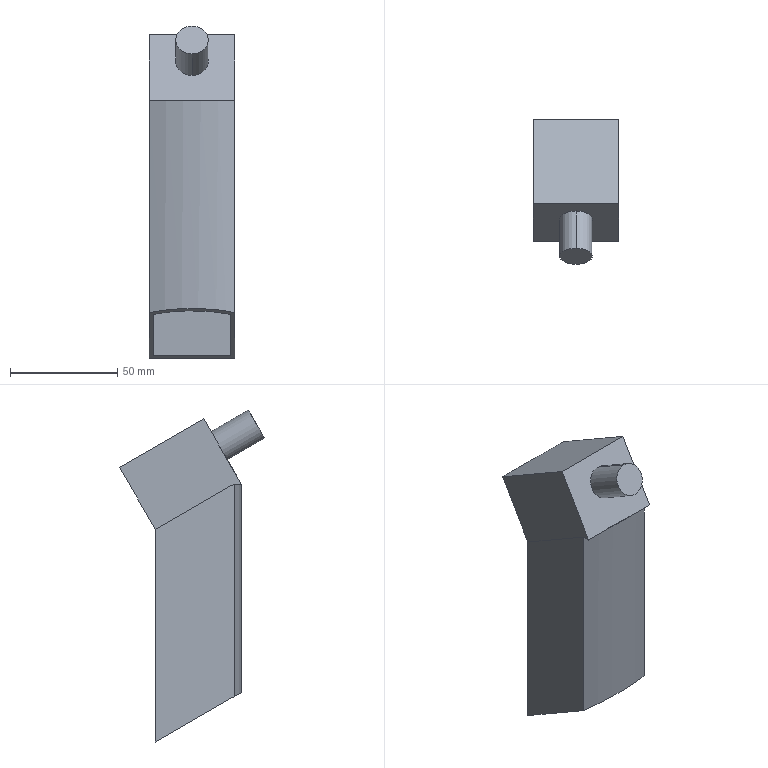Part | NX | 2 solids | 28 faces | box 40 x 67.338 x 154.471 mm | volume 46471 mm3 | plane 24 | cylinder 4 | commonest cylinder face diameters 15 x2 116 x1 120 x1
STEP:
#1=CARTESIAN_POINT('',(-12.806,-56.569,120.));
#2=VERTEX_POINT('',#1);
#3=CARTESIAN_POINT('',(-20.,-56.569,120.));
#4=VERTEX_POINT('',#3);
#5=CARTESIAN_POINT('',(25.,-56.569,120.));
#6=DIRECTION('',(-1.,0.,0.));
#7=VECTOR('',#6,1.);
#8=LINE('',#5,#7);
#9=EDGE_CURVE('',#2,#4,#8,.T.);
#10=ORIENTED_EDGE('',*,*,#9,.T.);
#11=CARTESIAN_POINT('',(20.,-56.569,120.));
#12=VERTEX_POINT('',#11);
#13=CARTESIAN_POINT('',(0.,0.,120.));
#14=DIRECTION('',(0.,0.,1.));
#15=DIRECTION('',(1.,0.,0.));
#16=AXIS2_PLACEMENT_3D('',#13,#14,#15);
#17=CIRCLE('',#16,60.);
#18=EDGE_CURVE('',#4,#12,#17,.T.);
#19=ORIENTED_EDGE('',*,*,#18,.T.);
#20=CARTESIAN_POINT('',(12.806,-56.569,120.));
#21=VERTEX_POINT('',#20);
#22=CARTESIAN_POINT('',(25.,-56.569,120.));
#23=DIRECTION('',(-1.,0.,0.));
#24=VECTOR('',#23,1.);
#25=LINE('',#22,#24);
#26=EDGE_CURVE('',#12,#21,#25,.T.);
#27=ORIENTED_EDGE('',*,*,#26,.T.);
#28=CARTESIAN_POINT('',(0.,0.,120.));
#29=DIRECTION('',(0.,0.,1.));
#30=DIRECTION('',(1.,0.,0.));
#31=AXIS2_PLACEMENT_3D('',#28,#29,#30);
#32=CIRCLE('',#31,58.);
#33=EDGE_CURVE('',#2,#21,#32,.T.);
#34=ORIENTED_EDGE('',*,*,#33,.F.);
#35=EDGE_LOOP('',(#10,#19,#27,#34));
#36=FACE_OUTER_BOUND('',#35,.T.);
#37=CARTESIAN_POINT('',(0.,0.,120.));
#38=DIRECTION('',(0.,0.,1.));
#39=DIRECTION('',(1.,0.,0.));
#40=AXIS2_PLACEMENT_3D('',#37,#38,#39);
#41=PLANE('',#40);
#42=ADVANCED_FACE('',(#36),#41,.T.);
#43=CARTESIAN_POINT('',(-20.,-56.569,21.113));
#44=VERTEX_POINT('',#43);
#45=CARTESIAN_POINT('',(-20.,-56.569,120.));
#46=DIRECTION('',(0.,0.,-1.));
#47=VECTOR('',#46,1.);
#48=LINE('',#45,#47);
#49=EDGE_CURVE('',#4,#44,#48,.T.);
#50=ORIENTED_EDGE('',*,*,#49,.T.);
#51=CARTESIAN_POINT('',(20.,-56.569,21.113));
#52=VERTEX_POINT('',#51);
#53=CARTESIAN_POINT('',(-20.,-56.569,21.113));
#54=CARTESIAN_POINT('',(-6.931,-61.189,23.781));
#55=CARTESIAN_POINT('',(6.931,-61.189,23.781));
#56=CARTESIAN_POINT('',(20.,-56.569,21.113));
#57=(BOUNDED_CURVE()B_SPLINE_CURVE(3,(#53,#54,#55,#56),.UNSPECIFIED.,.F.,.F.)B_SPLINE_CURVE_WITH_KNOTS((4,4),(0.,1.),.UNSPECIFIED.)CURVE()GEOMETRIC_REPRESENTATION_ITEM()RATIONAL_B_SPLINE_CURVE((1.,0.9619,0.9619,1.))REPRESENTATION_ITEM(''));
#58=EDGE_CURVE('',#44,#52,#57,.T.);
#59=ORIENTED_EDGE('',*,*,#58,.T.);
#60=CARTESIAN_POINT('',(20.,-56.569,120.));
#61=DIRECTION('',(0.,0.,-1.));
#62=VECTOR('',#61,1.);
#63=LINE('',#60,#62);
#64=EDGE_CURVE('',#12,#52,#63,.T.);
#65=ORIENTED_EDGE('',*,*,#64,.F.);
#66=ORIENTED_EDGE('',*,*,#18,.F.);
#67=EDGE_LOOP('',(#50,#59,#65,#66));
#68=FACE_OUTER_BOUND('',#67,.T.);
#69=CARTESIAN_POINT('',(0.,0.,120.));
#70=DIRECTION('',(0.,0.,-1.));
#71=DIRECTION('',(-1.,0.,0.));
#72=AXIS2_PLACEMENT_3D('',#69,#70,#71);
#73=CYLINDRICAL_SURFACE('',#72,60.);
#74=ADVANCED_FACE('',(#68),#73,.T.);
#75=CARTESIAN_POINT('',(20.,-20.,98.887));
#76=VERTEX_POINT('',#75);
#77=CARTESIAN_POINT('',(20.,-20.,0.));
#78=VERTEX_POINT('',#77);
#79=CARTESIAN_POINT('',(20.,-20.,120.));
#80=DIRECTION('',(0.,0.,-1.));
#81=VECTOR('',#80,1.);
#82=LINE('',#79,#81);
#83=EDGE_CURVE('',#76,#78,#82,.T.);
#84=ORIENTED_EDGE('',*,*,#83,.F.);
#85=CARTESIAN_POINT('',(20.,-56.569,120.));
#86=DIRECTION('',(0.,-0.866,0.5));
#87=VECTOR('',#86,1.);
#88=LINE('',#85,#87);
#89=EDGE_CURVE('',#76,#12,#88,.T.);
#90=ORIENTED_EDGE('',*,*,#89,.T.);
#91=ORIENTED_EDGE('',*,*,#64,.T.);
#92=CARTESIAN_POINT('',(20.,-60.,23.094));
#93=DIRECTION('',(0.,0.866,-0.5));
#94=VECTOR('',#93,1.);
#95=LINE('',#92,#94);
#96=EDGE_CURVE('',#52,#78,#95,.T.);
#97=ORIENTED_EDGE('',*,*,#96,.T.);
#98=EDGE_LOOP('',(#84,#90,#91,#97));
#99=FACE_OUTER_BOUND('',#98,.T.);
#100=CARTESIAN_POINT('',(20.,-56.569,120.));
#101=DIRECTION('',(-1.,0.,0.));
#102=DIRECTION('',(0.,0.,1.));
#103=AXIS2_PLACEMENT_3D('',#100,#101,#102);
#104=PLANE('',#103);
#105=ADVANCED_FACE('',(#99),#104,.F.);
#106=CARTESIAN_POINT('',(-20.,-20.,98.887));
#107=VERTEX_POINT('',#106);
#108=CARTESIAN_POINT('',(-20.,-20.,0.));
#109=VERTEX_POINT('',#108);
#110=CARTESIAN_POINT('',(-20.,-20.,120.));
#111=DIRECTION('',(0.,0.,-1.));
#112=VECTOR('',#111,1.);
#113=LINE('',#110,#112);
#114=EDGE_CURVE('',#107,#109,#113,.T.);
#115=ORIENTED_EDGE('',*,*,#114,.F.);
#116=CARTESIAN_POINT('',(25.,-20.,98.887));
#117=DIRECTION('',(-1.,0.,0.));
#118=VECTOR('',#117,1.);
#119=LINE('',#116,#118);
#120=EDGE_CURVE('',#76,#107,#119,.T.);
#121=ORIENTED_EDGE('',*,*,#120,.F.);
#122=ORIENTED_EDGE('',*,*,#83,.T.);
#123=CARTESIAN_POINT('',(-20.,-20.,0.));
#124=DIRECTION('',(-1.,0.,0.));
#125=VECTOR('',#124,1.);
#126=LINE('',#123,#125);
#127=EDGE_CURVE('',#78,#109,#126,.T.);
#128=ORIENTED_EDGE('',*,*,#127,.T.);
#129=EDGE_LOOP('',(#115,#121,#122,#128));
#130=FACE_OUTER_BOUND('',#129,.T.);
#131=CARTESIAN_POINT('',(-20.,-20.,120.));
#132=DIRECTION('',(0.,-1.,0.));
#133=DIRECTION('',(0.,0.,-1.));
#134=AXIS2_PLACEMENT_3D('',#131,#132,#133);
#135=PLANE('',#134);
#136=ADVANCED_FACE('',(#130),#135,.F.);
#137=ORIENTED_EDGE('',*,*,#49,.F.);
#138=CARTESIAN_POINT('',(-20.,-56.569,120.));
#139=DIRECTION('',(0.,-0.866,0.5));
#140=VECTOR('',#139,1.);
#141=LINE('',#138,#140);
#142=EDGE_CURVE('',#107,#4,#141,.T.);
#143=ORIENTED_EDGE('',*,*,#142,.F.);
#144=ORIENTED_EDGE('',*,*,#114,.T.);
#145=CARTESIAN_POINT('',(-20.,-60.,23.094));
#146=DIRECTION('',(0.,0.866,-0.5));
#147=VECTOR('',#146,1.);
#148=LINE('',#145,#147);
#149=EDGE_CURVE('',#44,#109,#148,.T.);
#150=ORIENTED_EDGE('',*,*,#149,.F.);
#151=EDGE_LOOP('',(#137,#143,#144,#150));
#152=FACE_OUTER_BOUND('',#151,.T.);
#153=CARTESIAN_POINT('',(-20.,-56.569,120.));
#154=DIRECTION('',(1.,0.,0.));
#155=DIRECTION('',(0.,0.,-1.));
#156=AXIS2_PLACEMENT_3D('',#153,#154,#155);
#157=PLANE('',#156);
#158=ADVANCED_FACE('',(#152),#157,.F.);
#159=CARTESIAN_POINT('',(-18.,-55.136,119.173));
#160=VERTEX_POINT('',#159);
#161=CARTESIAN_POINT('',(-18.,-22.,100.042));
#162=VERTEX_POINT('',#161);
#163=CARTESIAN_POINT('',(-18.,-55.494,119.38));
#164=DIRECTION('',(0.,0.866,-0.5));
#165=VECTOR('',#164,1.);
#166=LINE('',#163,#165);
#167=EDGE_CURVE('',#160,#162,#166,.T.);
#168=ORIENTED_EDGE('',*,*,#167,.F.);
#169=CARTESIAN_POINT('',(-18.,-55.136,20.286));
#170=VERTEX_POINT('',#169);
#171=CARTESIAN_POINT('',(-18.,-55.136,120.));
#172=DIRECTION('',(0.,0.,-1.));
#173=VECTOR('',#172,1.);
#174=LINE('',#171,#173);
#175=EDGE_CURVE('',#160,#170,#174,.T.);
#176=ORIENTED_EDGE('',*,*,#175,.T.);
#177=CARTESIAN_POINT('',(-18.,-22.,1.155));
#178=VERTEX_POINT('',#177);
#179=CARTESIAN_POINT('',(-18.,-98.314,45.214));
#180=DIRECTION('',(0.,-0.866,0.5));
#181=VECTOR('',#180,1.);
#182=LINE('',#179,#181);
#183=EDGE_CURVE('',#178,#170,#182,.T.);
#184=ORIENTED_EDGE('',*,*,#183,.F.);
#185=CARTESIAN_POINT('',(-18.,-22.,120.));
#186=DIRECTION('',(0.,0.,-1.));
#187=VECTOR('',#186,1.);
#188=LINE('',#185,#187);
#189=EDGE_CURVE('',#162,#178,#188,.T.);
#190=ORIENTED_EDGE('',*,*,#189,.F.);
#191=EDGE_LOOP('',(#168,#176,#184,#190));
#192=FACE_OUTER_BOUND('',#191,.T.);
#193=CARTESIAN_POINT('',(-18.,-55.136,120.));
#194=DIRECTION('',(1.,0.,0.));
#195=DIRECTION('',(0.,1.,0.));
#196=AXIS2_PLACEMENT_3D('',#193,#194,#195);
#197=PLANE('',#196);
#198=ADVANCED_FACE('',(#192),#197,.T.);
#199=CARTESIAN_POINT('',(18.,-55.136,119.173));
#200=VERTEX_POINT('',#199);
#201=CARTESIAN_POINT('',(18.,-55.136,119.173));
#202=CARTESIAN_POINT('',(16.292,-55.694,119.495));
#203=CARTESIAN_POINT('',(14.559,-56.172,119.771));
#204=CARTESIAN_POINT('',(12.806,-56.569,120.));
#205=(BOUNDED_CURVE()B_SPLINE_CURVE(3,(#201,#202,#203,#204),.UNSPECIFIED.,.F.,.F.)B_SPLINE_CURVE_WITH_KNOTS((4,4),(0.,1.),.UNSPECIFIED.)CURVE()GEOMETRIC_REPRESENTATION_ITEM()RATIONAL_B_SPLINE_CURVE((1.,0.9993,0.9993,1.))REPRESENTATION_ITEM(''));
#206=EDGE_CURVE('',#200,#21,#205,.T.);
#207=ORIENTED_EDGE('',*,*,#206,.F.);
#208=CARTESIAN_POINT('',(18.,-55.136,20.286));
#209=VERTEX_POINT('',#208);
#210=CARTESIAN_POINT('',(18.,-55.136,120.));
#211=DIRECTION('',(0.,0.,-1.));
#212=VECTOR('',#211,1.);
#213=LINE('',#210,#212);
#214=EDGE_CURVE('',#200,#209,#213,.T.);
#215=ORIENTED_EDGE('',*,*,#214,.T.);
#216=CARTESIAN_POINT('',(-18.,-55.136,20.286));
#217=CARTESIAN_POINT('',(-6.204,-58.987,22.509));
#218=CARTESIAN_POINT('',(6.204,-58.987,22.509));
#219=CARTESIAN_POINT('',(18.,-55.136,20.286));
#220=(BOUNDED_CURVE()B_SPLINE_CURVE(3,(#216,#217,#218,#219),.UNSPECIFIED.,.F.,.F.)B_SPLINE_CURVE_WITH_KNOTS((4,4),(0.,1.),.UNSPECIFIED.)CURVE()GEOMETRIC_REPRESENTATION_ITEM()RATIONAL_B_SPLINE_CURVE((1.,0.9671,0.9671,1.))REPRESENTATION_ITEM(''));
#221=EDGE_CURVE('',#170,#209,#220,.T.);
#222=ORIENTED_EDGE('',*,*,#221,.F.);
#223=ORIENTED_EDGE('',*,*,#175,.F.);
#224=CARTESIAN_POINT('',(-12.806,-56.569,120.));
#225=CARTESIAN_POINT('',(-14.559,-56.172,119.771));
#226=CARTESIAN_POINT('',(-16.292,-55.694,119.495));
#227=CARTESIAN_POINT('',(-18.,-55.136,119.173));
#228=(BOUNDED_CURVE()B_SPLINE_CURVE(3,(#224,#225,#226,#227),.UNSPECIFIED.,.F.,.F.)B_SPLINE_CURVE_WITH_KNOTS((4,4),(0.,1.),.UNSPECIFIED.)CURVE()GEOMETRIC_REPRESENTATION_ITEM()RATIONAL_B_SPLINE_CURVE((1.,0.9993,0.9993,1.))REPRESENTATION_ITEM(''));
#229=EDGE_CURVE('',#2,#160,#228,.T.);
#230=ORIENTED_EDGE('',*,*,#229,.F.);
#231=ORIENTED_EDGE('',*,*,#33,.T.);
#232=EDGE_LOOP('',(#207,#215,#222,#223,#230,#231));
#233=FACE_OUTER_BOUND('',#232,.T.);
#234=CARTESIAN_POINT('',(0.,0.,120.));
#235=DIRECTION('',(0.,0.,-1.));
#236=DIRECTION('',(-1.,0.,0.));
#237=AXIS2_PLACEMENT_3D('',#234,#235,#236);
#238=CYLINDRICAL_SURFACE('',#237,58.);
#239=ADVANCED_FACE('',(#233),#238,.F.);
#240=CARTESIAN_POINT('',(18.,-22.,100.042));
#241=VERTEX_POINT('',#240);
#242=CARTESIAN_POINT('',(18.,-55.494,119.38));
#243=DIRECTION('',(0.,-0.866,0.5));
#244=VECTOR('',#243,1.);
#245=LINE('',#242,#244);
#246=EDGE_CURVE('',#241,#200,#245,.T.);
#247=ORIENTED_EDGE('',*,*,#246,.F.);
#248=CARTESIAN_POINT('',(18.,-22.,1.155));
#249=VERTEX_POINT('',#248);
#250=CARTESIAN_POINT('',(18.,-22.,120.));
#251=DIRECTION('',(0.,0.,-1.));
#252=VECTOR('',#251,1.);
#253=LINE('',#250,#252);
#254=EDGE_CURVE('',#241,#249,#253,.T.);
#255=ORIENTED_EDGE('',*,*,#254,.T.);
#256=CARTESIAN_POINT('',(18.,-98.314,45.214));
#257=DIRECTION('',(0.,0.866,-0.5));
#258=VECTOR('',#257,1.);
#259=LINE('',#256,#258);
#260=EDGE_CURVE('',#209,#249,#259,.T.);
#261=ORIENTED_EDGE('',*,*,#260,.F.);
#262=ORIENTED_EDGE('',*,*,#214,.F.);
#263=EDGE_LOOP('',(#247,#255,#261,#262));
#264=FACE_OUTER_BOUND('',#263,.T.);
#265=CARTESIAN_POINT('',(18.,-55.136,120.));
#266=DIRECTION('',(-1.,0.,0.));
#267=DIRECTION('',(0.,-1.,0.));
#268=AXIS2_PLACEMENT_3D('',#265,#266,#267);
#269=PLANE('',#268);
#270=ADVANCED_FACE('',(#264),#269,.T.);
#271=CARTESIAN_POINT('',(-18.,-22.,100.042));
#272=DIRECTION('',(1.,0.,0.));
#273=VECTOR('',#272,1.);
#274=LINE('',#271,#273);
#275=EDGE_CURVE('',#162,#241,#274,.T.);
#276=ORIENTED_EDGE('',*,*,#275,.F.);
#277=ORIENTED_EDGE('',*,*,#189,.T.);
#278=CARTESIAN_POINT('',(-18.,-22.,1.155));
#279=DIRECTION('',(-1.,0.,0.));
#280=VECTOR('',#279,1.);
#281=LINE('',#278,#280);
#282=EDGE_CURVE('',#249,#178,#281,.T.);
#283=ORIENTED_EDGE('',*,*,#282,.F.);
#284=ORIENTED_EDGE('',*,*,#254,.F.);
#285=EDGE_LOOP('',(#276,#277,#283,#284));
#286=FACE_OUTER_BOUND('',#285,.T.);
#287=CARTESIAN_POINT('',(-18.,-22.,120.));
#288=DIRECTION('',(0.,-1.,0.));
#289=DIRECTION('',(0.,0.,-1.));
#290=AXIS2_PLACEMENT_3D('',#287,#288,#289);
#291=PLANE('',#290);
#292=ADVANCED_FACE('',(#286),#291,.T.);
#293=ORIENTED_EDGE('',*,*,#183,.T.);
#294=ORIENTED_EDGE('',*,*,#221,.T.);
#295=ORIENTED_EDGE('',*,*,#260,.T.);
#296=ORIENTED_EDGE('',*,*,#282,.T.);
#297=EDGE_LOOP('',(#293,#294,#295,#296));
#298=FACE_BOUND('',#297,.T.);
#299=ORIENTED_EDGE('',*,*,#149,.T.);
#300=ORIENTED_EDGE('',*,*,#127,.F.);
#301=ORIENTED_EDGE('',*,*,#96,.F.);
#302=ORIENTED_EDGE('',*,*,#58,.F.);
#303=EDGE_LOOP('',(#299,#300,#301,#302));
#304=FACE_BOUND('',#303,.T.);
#305=CARTESIAN_POINT('',(20.,-60.,23.094));
#306=DIRECTION('',(0.,0.5,0.866));
#307=DIRECTION('',(0.,-0.866,0.5));
#308=AXIS2_PLACEMENT_3D('',#305,#306,#307);
#309=PLANE('',#308);
#310=ADVANCED_FACE('',(#298,#304),#309,.F.);
#311=ORIENTED_EDGE('',*,*,#120,.T.);
#312=ORIENTED_EDGE('',*,*,#142,.T.);
#313=ORIENTED_EDGE('',*,*,#9,.F.);
#314=ORIENTED_EDGE('',*,*,#229,.T.);
#315=ORIENTED_EDGE('',*,*,#167,.T.);
#316=ORIENTED_EDGE('',*,*,#275,.T.);
#317=ORIENTED_EDGE('',*,*,#246,.T.);
#318=ORIENTED_EDGE('',*,*,#206,.T.);
#319=ORIENTED_EDGE('',*,*,#26,.F.);
#320=ORIENTED_EDGE('',*,*,#89,.F.);
#321=EDGE_LOOP('',(#311,#312,#313,#314,#315,#316,#317,#318,#319,#320));
#322=FACE_OUTER_BOUND('',#321,.T.);
#323=CARTESIAN_POINT('',(25.,-56.569,120.));
#324=DIRECTION('',(0.,-0.5,-0.866));
#325=DIRECTION('',(0.,0.866,-0.5));
#326=AXIS2_PLACEMENT_3D('',#323,#324,#325);
#327=PLANE('',#326);
#328=ADVANCED_FACE('',(#322),#327,.F.);
#329=CLOSED_SHELL('',(#42,#74,#105,#136,#158,#198,#239,#270,#292,#310,#328));
#330=MANIFOLD_SOLID_BREP('',#329);
#331=CARTESIAN_POINT('',(0.,-70.692,141.481));
#332=VERTEX_POINT('',#331);
#333=CARTESIAN_POINT('',(0.,-63.192,154.471));
#334=VERTEX_POINT('',#333);
#335=CARTESIAN_POINT('',(0.,-66.942,147.976));
#336=DIRECTION('',(0.,-0.866,0.5));
#337=DIRECTION('',(0.,-0.5,-0.866));
#338=AXIS2_PLACEMENT_3D('',#335,#336,#337);
#339=CIRCLE('',#338,7.5);
#340=EDGE_CURVE('',#332,#334,#339,.T.);
#341=ORIENTED_EDGE('',*,*,#340,.F.);
#342=CARTESIAN_POINT('',(0.,-53.371,131.481));
#343=VERTEX_POINT('',#342);
#344=CARTESIAN_POINT('',(0.,-70.692,141.481));
#345=DIRECTION('',(0.,0.866,-0.5));
#346=VECTOR('',#345,1.);
#347=LINE('',#344,#346);
#348=EDGE_CURVE('',#332,#343,#347,.T.);
#349=ORIENTED_EDGE('',*,*,#348,.T.);
#350=CARTESIAN_POINT('',(0.,-45.871,144.471));
#351=VERTEX_POINT('',#350);
#352=CARTESIAN_POINT('',(0.,-49.621,137.976));
#353=DIRECTION('',(0.,-0.866,0.5));
#354=DIRECTION('',(0.,-0.5,-0.866));
#355=AXIS2_PLACEMENT_3D('',#352,#353,#354);
#356=CIRCLE('',#355,7.5);
#357=EDGE_CURVE('',#343,#351,#356,.T.);
#358=ORIENTED_EDGE('',*,*,#357,.T.);
#359=CARTESIAN_POINT('',(0.,-63.192,154.471));
#360=DIRECTION('',(0.,0.866,-0.5));
#361=VECTOR('',#360,1.);
#362=LINE('',#359,#361);
#363=EDGE_CURVE('',#334,#351,#362,.T.);
#364=ORIENTED_EDGE('',*,*,#363,.F.);
#365=EDGE_LOOP('',(#341,#349,#358,#364));
#366=FACE_OUTER_BOUND('',#365,.T.);
#367=CARTESIAN_POINT('',(0.,-66.942,147.976));
#368=DIRECTION('',(0.,0.866,-0.5));
#369=DIRECTION('',(0.,0.5,0.866));
#370=AXIS2_PLACEMENT_3D('',#367,#368,#369);
#371=CYLINDRICAL_SURFACE('',#370,7.5);
#372=ADVANCED_FACE('',(#366),#371,.T.);
#373=CARTESIAN_POINT('',(20.,-42.5,150.311));
#374=VERTEX_POINT('',#373);
#375=CARTESIAN_POINT('',(20.,-60.,120.));
#376=VERTEX_POINT('',#375);
#377=CARTESIAN_POINT('',(20.,-60.,120.));
#378=DIRECTION('',(0.,-0.5,-0.866));
#379=VECTOR('',#378,1.);
#380=LINE('',#377,#379);
#381=EDGE_CURVE('',#374,#376,#380,.T.);
#382=ORIENTED_EDGE('',*,*,#381,.F.);
#383=CARTESIAN_POINT('',(-20.,-42.5,150.311));
#384=VERTEX_POINT('',#383);
#385=CARTESIAN_POINT('',(-20.,-42.5,150.311));
#386=DIRECTION('',(1.,0.,0.));
#387=VECTOR('',#386,1.);
#388=LINE('',#385,#387);
#389=EDGE_CURVE('',#384,#374,#388,.T.);
#390=ORIENTED_EDGE('',*,*,#389,.F.);
#391=CARTESIAN_POINT('',(-20.,-60.,120.));
#392=VERTEX_POINT('',#391);
#393=CARTESIAN_POINT('',(-20.,-60.,120.));
#394=DIRECTION('',(0.,-0.5,-0.866));
#395=VECTOR('',#394,1.);
#396=LINE('',#393,#395);
#397=EDGE_CURVE('',#384,#392,#396,.T.);
#398=ORIENTED_EDGE('',*,*,#397,.T.);
#399=CARTESIAN_POINT('',(-20.,-60.,120.));
#400=DIRECTION('',(1.,0.,0.));
#401=VECTOR('',#400,1.);
#402=LINE('',#399,#401);
#403=EDGE_CURVE('',#392,#376,#402,.T.);
#404=ORIENTED_EDGE('',*,*,#403,.T.);
#405=EDGE_LOOP('',(#382,#390,#398,#404));
#406=FACE_BOUND('',#405,.T.);
#407=CARTESIAN_POINT('',(0.,-49.621,137.976));
#408=DIRECTION('',(0.,-0.866,0.5));
#409=DIRECTION('',(0.,-0.5,-0.866));
#410=AXIS2_PLACEMENT_3D('',#407,#408,#409);
#411=CIRCLE('',#410,7.5);
#412=EDGE_CURVE('',#351,#343,#411,.T.);
#413=ORIENTED_EDGE('',*,*,#412,.F.);
#414=ORIENTED_EDGE('',*,*,#357,.F.);
#415=EDGE_LOOP('',(#413,#414));
#416=FACE_BOUND('',#415,.T.);
#417=CARTESIAN_POINT('',(-20.,-60.,120.));
#418=DIRECTION('',(0.,-0.866,0.5));
#419=DIRECTION('',(0.,-0.5,-0.866));
#420=AXIS2_PLACEMENT_3D('',#417,#418,#419);
#421=PLANE('',#420);
#422=ADVANCED_FACE('',(#406,#416),#421,.T.);
#423=CARTESIAN_POINT('',(-18.,-41.768,147.579));
#424=VERTEX_POINT('',#423);
#425=CARTESIAN_POINT('',(18.,-41.768,147.579));
#426=VERTEX_POINT('',#425);
#427=CARTESIAN_POINT('',(-20.,-41.768,147.579));
#428=DIRECTION('',(1.,0.,0.));
#429=VECTOR('',#428,1.);
#430=LINE('',#427,#429);
#431=EDGE_CURVE('',#424,#426,#430,.T.);
#432=ORIENTED_EDGE('',*,*,#431,.F.);
#433=CARTESIAN_POINT('',(-18.,-6.086,126.978));
#434=VERTEX_POINT('',#433);
#435=CARTESIAN_POINT('',(-18.,-40.926,147.093));
#436=DIRECTION('',(0.,-0.866,0.5));
#437=VECTOR('',#436,1.);
#438=LINE('',#435,#437);
#439=EDGE_CURVE('',#434,#424,#438,.T.);
#440=ORIENTED_EDGE('',*,*,#439,.F.);
#441=CARTESIAN_POINT('',(18.,-6.086,126.978));
#442=VERTEX_POINT('',#441);
#443=CARTESIAN_POINT('',(-20.,-6.086,126.978));
#444=DIRECTION('',(1.,0.,0.));
#445=VECTOR('',#444,1.);
#446=LINE('',#443,#445);
#447=EDGE_CURVE('',#434,#442,#446,.T.);
#448=ORIENTED_EDGE('',*,*,#447,.T.);
#449=CARTESIAN_POINT('',(18.,-40.926,147.093));
#450=DIRECTION('',(0.,-0.866,0.5));
#451=VECTOR('',#450,1.);
#452=LINE('',#449,#451);
#453=EDGE_CURVE('',#442,#426,#452,.T.);
#454=ORIENTED_EDGE('',*,*,#453,.T.);
#455=EDGE_LOOP('',(#432,#440,#448,#454));
#456=FACE_OUTER_BOUND('',#455,.T.);
#457=CARTESIAN_POINT('',(-20.,-40.926,147.093));
#458=DIRECTION('',(0.,0.5,0.866));
#459=DIRECTION('',(0.,-0.866,0.5));
#460=AXIS2_PLACEMENT_3D('',#457,#458,#459);
#461=PLANE('',#460);
#462=ADVANCED_FACE('',(#456),#461,.F.);
#463=CARTESIAN_POINT('',(18.,-56.569,120.));
#464=VERTEX_POINT('',#463);
#465=CARTESIAN_POINT('',(20.,-56.569,120.));
#466=VERTEX_POINT('',#465);
#467=CARTESIAN_POINT('',(25.,-56.569,120.));
#468=DIRECTION('',(1.,0.,0.));
#469=VECTOR('',#468,1.);
#470=LINE('',#467,#469);
#471=EDGE_CURVE('',#464,#466,#470,.T.);
#472=ORIENTED_EDGE('',*,*,#471,.F.);
#473=CARTESIAN_POINT('',(18.,-21.728,99.885));
#474=VERTEX_POINT('',#473);
#475=CARTESIAN_POINT('',(18.,-56.569,120.));
#476=DIRECTION('',(0.,0.866,-0.5));
#477=VECTOR('',#476,1.);
#478=LINE('',#475,#477);
#479=EDGE_CURVE('',#464,#474,#478,.T.);
#480=ORIENTED_EDGE('',*,*,#479,.T.);
#481=CARTESIAN_POINT('',(-18.,-21.728,99.885));
#482=VERTEX_POINT('',#481);
#483=CARTESIAN_POINT('',(25.,-21.728,99.885));
#484=DIRECTION('',(1.,0.,0.));
#485=VECTOR('',#484,1.);
#486=LINE('',#483,#485);
#487=EDGE_CURVE('',#482,#474,#486,.T.);
#488=ORIENTED_EDGE('',*,*,#487,.F.);
#489=CARTESIAN_POINT('',(-18.,-56.569,120.));
#490=VERTEX_POINT('',#489);
#491=CARTESIAN_POINT('',(-18.,-56.569,120.));
#492=DIRECTION('',(0.,0.866,-0.5));
#493=VECTOR('',#492,1.);
#494=LINE('',#491,#493);
#495=EDGE_CURVE('',#490,#482,#494,.T.);
#496=ORIENTED_EDGE('',*,*,#495,.F.);
#497=CARTESIAN_POINT('',(-20.,-56.569,120.));
#498=VERTEX_POINT('',#497);
#499=CARTESIAN_POINT('',(-20.,-56.569,120.));
#500=DIRECTION('',(1.,0.,0.));
#501=VECTOR('',#500,1.);
#502=LINE('',#499,#501);
#503=EDGE_CURVE('',#498,#490,#502,.T.);
#504=ORIENTED_EDGE('',*,*,#503,.F.);
#505=CARTESIAN_POINT('',(-20.,-19.996,98.885));
#506=VERTEX_POINT('',#505);
#507=CARTESIAN_POINT('',(-20.,-56.569,120.));
#508=DIRECTION('',(0.,0.866,-0.5));
#509=VECTOR('',#508,1.);
#510=LINE('',#507,#509);
#511=EDGE_CURVE('',#498,#506,#510,.T.);
#512=ORIENTED_EDGE('',*,*,#511,.T.);
#513=CARTESIAN_POINT('',(20.,-19.996,98.885));
#514=VERTEX_POINT('',#513);
#515=CARTESIAN_POINT('',(25.,-19.996,98.885));
#516=DIRECTION('',(1.,0.,0.));
#517=VECTOR('',#516,1.);
#518=LINE('',#515,#517);
#519=EDGE_CURVE('',#506,#514,#518,.T.);
#520=ORIENTED_EDGE('',*,*,#519,.T.);
#521=CARTESIAN_POINT('',(20.,-56.569,120.));
#522=DIRECTION('',(0.,0.866,-0.5));
#523=VECTOR('',#522,1.);
#524=LINE('',#521,#523);
#525=EDGE_CURVE('',#466,#514,#524,.T.);
#526=ORIENTED_EDGE('',*,*,#525,.F.);
#527=EDGE_LOOP('',(#472,#480,#488,#496,#504,#512,#520,#526));
#528=FACE_OUTER_BOUND('',#527,.T.);
#529=CARTESIAN_POINT('',(25.,-56.569,120.));
#530=DIRECTION('',(0.,-0.5,-0.866));
#531=DIRECTION('',(0.,0.866,-0.5));
#532=AXIS2_PLACEMENT_3D('',#529,#530,#531);
#533=PLANE('',#532);
#534=ADVANCED_FACE('',(#528),#533,.T.);
#535=CARTESIAN_POINT('',(20.,-3.354,127.71));
#536=VERTEX_POINT('',#535);
#537=CARTESIAN_POINT('',(20.,-39.926,148.825));
#538=DIRECTION('',(0.,-0.866,0.5));
#539=VECTOR('',#538,1.);
#540=LINE('',#537,#539);
#541=EDGE_CURVE('',#536,#374,#540,.T.);
#542=ORIENTED_EDGE('',*,*,#541,.F.);
#543=CARTESIAN_POINT('',(-20.,-3.354,127.71));
#544=VERTEX_POINT('',#543);
#545=CARTESIAN_POINT('',(-20.,-3.354,127.71));
#546=DIRECTION('',(1.,0.,0.));
#547=VECTOR('',#546,1.);
#548=LINE('',#545,#547);
#549=EDGE_CURVE('',#544,#536,#548,.T.);
#550=ORIENTED_EDGE('',*,*,#549,.F.);
#551=CARTESIAN_POINT('',(-20.,-39.926,148.825));
#552=DIRECTION('',(0.,-0.866,0.5));
#553=VECTOR('',#552,1.);
#554=LINE('',#551,#553);
#555=EDGE_CURVE('',#544,#384,#554,.T.);
#556=ORIENTED_EDGE('',*,*,#555,.T.);
#557=ORIENTED_EDGE('',*,*,#389,.T.);
#558=EDGE_LOOP('',(#542,#550,#556,#557));
#559=FACE_OUTER_BOUND('',#558,.T.);
#560=CARTESIAN_POINT('',(-20.,-39.926,148.825));
#561=DIRECTION('',(0.,0.5,0.866));
#562=DIRECTION('',(0.,-0.866,0.5));
#563=AXIS2_PLACEMENT_3D('',#560,#561,#562);
#564=PLANE('',#563);
#565=ADVANCED_FACE('',(#559),#564,.T.);
#566=CARTESIAN_POINT('',(20.,-3.354,127.71));
#567=DIRECTION('',(0.,0.5,0.866));
#568=VECTOR('',#567,1.);
#569=LINE('',#566,#568);
#570=EDGE_CURVE('',#514,#536,#569,.T.);
#571=ORIENTED_EDGE('',*,*,#570,.F.);
#572=ORIENTED_EDGE('',*,*,#519,.F.);
#573=CARTESIAN_POINT('',(-20.,-3.354,127.71));
#574=DIRECTION('',(0.,0.5,0.866));
#575=VECTOR('',#574,1.);
#576=LINE('',#573,#575);
#577=EDGE_CURVE('',#506,#544,#576,.T.);
#578=ORIENTED_EDGE('',*,*,#577,.T.);
#579=ORIENTED_EDGE('',*,*,#549,.T.);
#580=EDGE_LOOP('',(#571,#572,#578,#579));
#581=FACE_OUTER_BOUND('',#580,.T.);
#582=CARTESIAN_POINT('',(-20.,-3.354,127.71));
#583=DIRECTION('',(0.,0.866,-0.5));
#584=DIRECTION('',(0.,0.5,0.866));
#585=AXIS2_PLACEMENT_3D('',#582,#583,#584);
#586=PLANE('',#585);
#587=ADVANCED_FACE('',(#581),#586,.T.);
#588=CARTESIAN_POINT('',(18.,-54.169,124.156));
#589=VERTEX_POINT('',#588);
#590=CARTESIAN_POINT('',(18.,-39.926,148.825));
#591=DIRECTION('',(0.,-0.5,-0.866));
#592=VECTOR('',#591,1.);
#593=LINE('',#590,#592);
#594=EDGE_CURVE('',#589,#464,#593,.T.);
#595=ORIENTED_EDGE('',*,*,#594,.T.);
#596=CARTESIAN_POINT('',(-20.,-56.569,120.));
#597=DIRECTION('',(1.,0.,0.));
#598=VECTOR('',#597,1.);
#599=LINE('',#596,#598);
#600=EDGE_CURVE('',#490,#464,#599,.T.);
#601=ORIENTED_EDGE('',*,*,#600,.F.);
#602=CARTESIAN_POINT('',(-18.,-54.169,124.156));
#603=VERTEX_POINT('',#602);
#604=CARTESIAN_POINT('',(-18.,-39.926,148.825));
#605=DIRECTION('',(0.,-0.5,-0.866));
#606=VECTOR('',#605,1.);
#607=LINE('',#604,#606);
#608=EDGE_CURVE('',#603,#490,#607,.T.);
#609=ORIENTED_EDGE('',*,*,#608,.F.);
#610=CARTESIAN_POINT('',(-20.,-54.169,124.156));
#611=DIRECTION('',(1.,0.,0.));
#612=VECTOR('',#611,1.);
#613=LINE('',#610,#612);
#614=EDGE_CURVE('',#603,#589,#613,.T.);
#615=ORIENTED_EDGE('',*,*,#614,.T.);
#616=EDGE_LOOP('',(#595,#601,#609,#615));
#617=FACE_OUTER_BOUND('',#616,.T.);
#618=CARTESIAN_POINT('',(-20.,-55.329,122.146));
#619=DIRECTION('',(0.,0.866,-0.5));
#620=DIRECTION('',(0.,0.5,0.866));
#621=AXIS2_PLACEMENT_3D('',#618,#619,#620);
#622=PLANE('',#621);
#623=ADVANCED_FACE('',(#617),#622,.T.);
#624=CARTESIAN_POINT('',(20.,-56.569,120.));
#625=DIRECTION('',(0.,1.,0.));
#626=VECTOR('',#625,1.);
#627=LINE('',#624,#626);
#628=EDGE_CURVE('',#376,#466,#627,.T.);
#629=ORIENTED_EDGE('',*,*,#628,.F.);
#630=ORIENTED_EDGE('',*,*,#403,.F.);
#631=CARTESIAN_POINT('',(-20.,-56.569,120.));
#632=DIRECTION('',(0.,1.,0.));
#633=VECTOR('',#632,1.);
#634=LINE('',#631,#633);
#635=EDGE_CURVE('',#392,#498,#634,.T.);
#636=ORIENTED_EDGE('',*,*,#635,.T.);
#637=ORIENTED_EDGE('',*,*,#503,.T.);
#638=ORIENTED_EDGE('',*,*,#600,.T.);
#639=ORIENTED_EDGE('',*,*,#471,.T.);
#640=EDGE_LOOP('',(#629,#630,#636,#637,#638,#639));
#641=FACE_OUTER_BOUND('',#640,.T.);
#642=CARTESIAN_POINT('',(-20.,-56.569,120.));
#643=DIRECTION('',(0.,0.,-1.));
#644=DIRECTION('',(-1.,0.,0.));
#645=AXIS2_PLACEMENT_3D('',#642,#643,#644);
#646=PLANE('',#645);
#647=ADVANCED_FACE('',(#641),#646,.T.);
#648=ORIENTED_EDGE('',*,*,#555,.F.);
#649=ORIENTED_EDGE('',*,*,#577,.F.);
#650=ORIENTED_EDGE('',*,*,#511,.F.);
#651=ORIENTED_EDGE('',*,*,#635,.F.);
#652=ORIENTED_EDGE('',*,*,#397,.F.);
#653=EDGE_LOOP('',(#648,#649,#650,#651,#652));
#654=FACE_OUTER_BOUND('',#653,.T.);
#655=CARTESIAN_POINT('',(-20.,-42.5,150.311));
#656=DIRECTION('',(-1.,0.,0.));
#657=DIRECTION('',(0.,0.,1.));
#658=AXIS2_PLACEMENT_3D('',#655,#656,#657);
#659=PLANE('',#658);
#660=ADVANCED_FACE('',(#654),#659,.T.);
#661=ORIENTED_EDGE('',*,*,#541,.T.);
#662=ORIENTED_EDGE('',*,*,#381,.T.);
#663=ORIENTED_EDGE('',*,*,#628,.T.);
#664=ORIENTED_EDGE('',*,*,#525,.T.);
#665=ORIENTED_EDGE('',*,*,#570,.T.);
#666=EDGE_LOOP('',(#661,#662,#663,#664,#665));
#667=FACE_OUTER_BOUND('',#666,.T.);
#668=CARTESIAN_POINT('',(20.,-42.5,150.311));
#669=DIRECTION('',(-1.,0.,0.));
#670=DIRECTION('',(0.,0.,1.));
#671=AXIS2_PLACEMENT_3D('',#668,#669,#670);
#672=PLANE('',#671);
#673=ADVANCED_FACE('',(#667),#672,.F.);
#674=CARTESIAN_POINT('',(-18.,-55.011,124.641));
#675=VERTEX_POINT('',#674);
#676=CARTESIAN_POINT('',(-18.,-17.597,103.041));
#677=DIRECTION('',(0.,0.866,-0.5));
#678=VECTOR('',#677,1.);
#679=LINE('',#676,#678);
#680=EDGE_CURVE('',#675,#603,#679,.T.);
#681=ORIENTED_EDGE('',*,*,#680,.F.);
#682=CARTESIAN_POINT('',(18.,-55.011,124.641));
#683=VERTEX_POINT('',#682);
#684=CARTESIAN_POINT('',(-20.,-55.011,124.641));
#685=DIRECTION('',(-1.,0.,0.));
#686=VECTOR('',#685,1.);
#687=LINE('',#684,#686);
#688=EDGE_CURVE('',#683,#675,#687,.T.);
#689=ORIENTED_EDGE('',*,*,#688,.F.);
#690=CARTESIAN_POINT('',(18.,-17.597,103.041));
#691=DIRECTION('',(0.,0.866,-0.5));
#692=VECTOR('',#691,1.);
#693=LINE('',#690,#692);
#694=EDGE_CURVE('',#683,#589,#693,.T.);
#695=ORIENTED_EDGE('',*,*,#694,.T.);
#696=ORIENTED_EDGE('',*,*,#614,.F.);
#697=EDGE_LOOP('',(#681,#689,#695,#696));
#698=FACE_OUTER_BOUND('',#697,.T.);
#699=CARTESIAN_POINT('',(-20.,-17.597,103.041));
#700=DIRECTION('',(0.,-0.5,-0.866));
#701=DIRECTION('',(0.,0.866,-0.5));
#702=AXIS2_PLACEMENT_3D('',#699,#700,#701);
#703=PLANE('',#702);
#704=ADVANCED_FACE('',(#698),#703,.F.);
#705=ORIENTED_EDGE('',*,*,#447,.F.);
#706=CARTESIAN_POINT('',(-18.,-5.086,128.71));
#707=DIRECTION('',(0.,0.5,0.866));
#708=VECTOR('',#707,1.);
#709=LINE('',#706,#708);
#710=EDGE_CURVE('',#482,#434,#709,.T.);
#711=ORIENTED_EDGE('',*,*,#710,.F.);
#712=ORIENTED_EDGE('',*,*,#487,.T.);
#713=CARTESIAN_POINT('',(18.,-5.086,128.71));
#714=DIRECTION('',(0.,0.5,0.866));
#715=VECTOR('',#714,1.);
#716=LINE('',#713,#715);
#717=EDGE_CURVE('',#474,#442,#716,.T.);
#718=ORIENTED_EDGE('',*,*,#717,.T.);
#719=EDGE_LOOP('',(#705,#711,#712,#718));
#720=FACE_OUTER_BOUND('',#719,.T.);
#721=CARTESIAN_POINT('',(-20.,-5.086,128.71));
#722=DIRECTION('',(0.,0.866,-0.5));
#723=DIRECTION('',(0.,0.5,0.866));
#724=AXIS2_PLACEMENT_3D('',#721,#722,#723);
#725=PLANE('',#724);
#726=ADVANCED_FACE('',(#720),#725,.F.);
#727=CARTESIAN_POINT('',(-18.,-58.268,119.));
#728=DIRECTION('',(0.,-0.5,-0.866));
#729=VECTOR('',#728,1.);
#730=LINE('',#727,#729);
#731=EDGE_CURVE('',#424,#675,#730,.T.);
#732=ORIENTED_EDGE('',*,*,#731,.F.);
#733=ORIENTED_EDGE('',*,*,#431,.T.);
#734=CARTESIAN_POINT('',(18.,-58.268,119.));
#735=DIRECTION('',(0.,-0.5,-0.866));
#736=VECTOR('',#735,1.);
#737=LINE('',#734,#736);
#738=EDGE_CURVE('',#426,#683,#737,.T.);
#739=ORIENTED_EDGE('',*,*,#738,.T.);
#740=ORIENTED_EDGE('',*,*,#688,.T.);
#741=EDGE_LOOP('',(#732,#733,#739,#740));
#742=FACE_OUTER_BOUND('',#741,.T.);
#743=CARTESIAN_POINT('',(-20.,-58.268,119.));
#744=DIRECTION('',(0.,-0.866,0.5));
#745=DIRECTION('',(0.,-0.5,-0.866));
#746=AXIS2_PLACEMENT_3D('',#743,#744,#745);
#747=PLANE('',#746);
#748=ADVANCED_FACE('',(#742),#747,.F.);
#749=ORIENTED_EDGE('',*,*,#439,.T.);
#750=ORIENTED_EDGE('',*,*,#731,.T.);
#751=ORIENTED_EDGE('',*,*,#680,.T.);
#752=ORIENTED_EDGE('',*,*,#608,.T.);
#753=ORIENTED_EDGE('',*,*,#495,.T.);
#754=ORIENTED_EDGE('',*,*,#710,.T.);
#755=EDGE_LOOP('',(#749,#750,#751,#752,#753,#754));
#756=FACE_OUTER_BOUND('',#755,.T.);
#757=CARTESIAN_POINT('',(-18.,-42.5,150.311));
#758=DIRECTION('',(-1.,0.,0.));
#759=DIRECTION('',(0.,0.,1.));
#760=AXIS2_PLACEMENT_3D('',#757,#758,#759);
#761=PLANE('',#760);
#762=ADVANCED_FACE('',(#756),#761,.F.);
#763=ORIENTED_EDGE('',*,*,#453,.F.);
#764=ORIENTED_EDGE('',*,*,#717,.F.);
#765=ORIENTED_EDGE('',*,*,#479,.F.);
#766=ORIENTED_EDGE('',*,*,#594,.F.);
#767=ORIENTED_EDGE('',*,*,#694,.F.);
#768=ORIENTED_EDGE('',*,*,#738,.F.);
#769=EDGE_LOOP('',(#763,#764,#765,#766,#767,#768));
#770=FACE_OUTER_BOUND('',#769,.T.);
#771=CARTESIAN_POINT('',(18.,-42.5,150.311));
#772=DIRECTION('',(-1.,0.,0.));
#773=DIRECTION('',(0.,0.,1.));
#774=AXIS2_PLACEMENT_3D('',#771,#772,#773);
#775=PLANE('',#774);
#776=ADVANCED_FACE('',(#770),#775,.T.);
#777=CARTESIAN_POINT('',(0.,-66.942,147.976));
#778=DIRECTION('',(0.,-0.866,0.5));
#779=DIRECTION('',(0.,-0.5,-0.866));
#780=AXIS2_PLACEMENT_3D('',#777,#778,#779);
#781=CIRCLE('',#780,7.5);
#782=EDGE_CURVE('',#334,#332,#781,.T.);
#783=ORIENTED_EDGE('',*,*,#782,.T.);
#784=ORIENTED_EDGE('',*,*,#340,.T.);
#785=EDGE_LOOP('',(#783,#784));
#786=FACE_OUTER_BOUND('',#785,.T.);
#787=CARTESIAN_POINT('',(0.,-66.942,147.976));
#788=DIRECTION('',(0.,-0.866,0.5));
#789=DIRECTION('',(0.,-0.5,-0.866));
#790=AXIS2_PLACEMENT_3D('',#787,#788,#789);
#791=PLANE('',#790);
#792=ADVANCED_FACE('',(#786),#791,.T.);
#793=ORIENTED_EDGE('',*,*,#348,.F.);
#794=ORIENTED_EDGE('',*,*,#782,.F.);
#795=ORIENTED_EDGE('',*,*,#363,.T.);
#796=ORIENTED_EDGE('',*,*,#412,.T.);
#797=EDGE_LOOP('',(#793,#794,#795,#796));
#798=FACE_OUTER_BOUND('',#797,.T.);
#799=CARTESIAN_POINT('',(0.,-66.942,147.976));
#800=DIRECTION('',(0.,0.866,-0.5));
#801=DIRECTION('',(0.,0.5,0.866));
#802=AXIS2_PLACEMENT_3D('',#799,#800,#801);
#803=CYLINDRICAL_SURFACE('',#802,7.5);
#804=ADVANCED_FACE('',(#798),#803,.T.);
#805=CLOSED_SHELL('',(#372,#422,#462,#534,#565,#587,#623,#647,#660,#673,#704,#726,#748,#762,#776,#792,#804));
#806=MANIFOLD_SOLID_BREP('',#805);
#807=(LENGTH_UNIT()NAMED_UNIT(*)SI_UNIT(.MILLI.,.METRE.));
#808=UNCERTAINTY_MEASURE_WITH_UNIT(LENGTH_MEASURE(0.00002),#807,'','');
#809=(NAMED_UNIT(*)PLANE_ANGLE_UNIT()SI_UNIT($,.RADIAN.));
#810=PLANE_ANGLE_MEASURE_WITH_UNIT(PLANE_ANGLE_MEASURE(0.01745),#809);
#811=DIMENSIONAL_EXPONENTS(0.,0.,0.,0.,0.,0.,0.);
#812=(CONVERSION_BASED_UNIT('DEGREE',#810)NAMED_UNIT(#811)PLANE_ANGLE_UNIT());
#813=(NAMED_UNIT(*)SI_UNIT($,.STERADIAN.)SOLID_ANGLE_UNIT());
#814=(GEOMETRIC_REPRESENTATION_CONTEXT(3)GLOBAL_UNCERTAINTY_ASSIGNED_CONTEXT((#808))GLOBAL_UNIT_ASSIGNED_CONTEXT((#807,#812,#813))REPRESENTATION_CONTEXT('',''));
#815=ADVANCED_BREP_SHAPE_REPRESENTATION('',(#330,#806),#814);